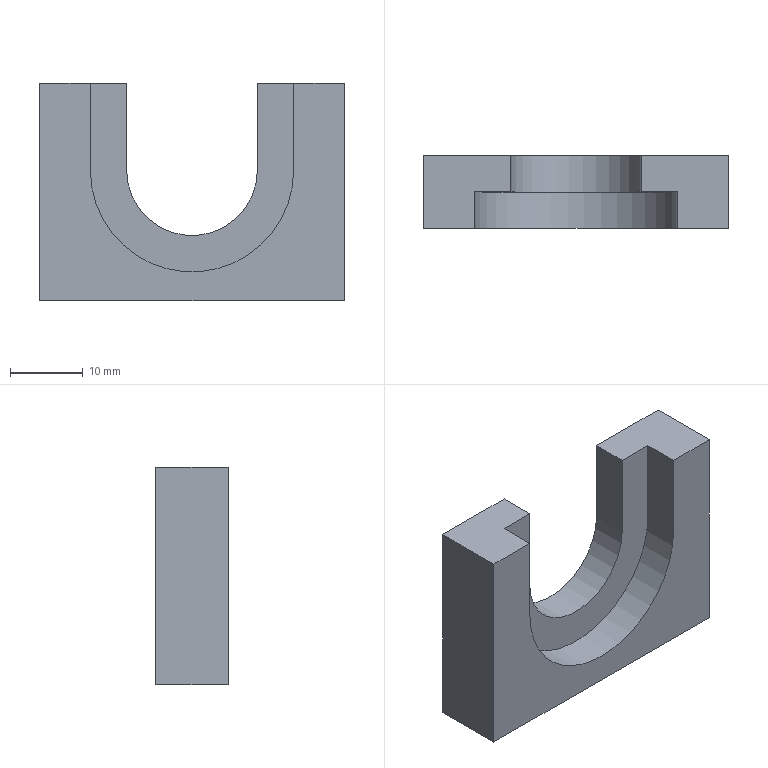Part | NX | features M5 六角凹头螺钉的柱形沉头孔1 2 | 1 solid | 14 faces | box 42 x 10 x 30 mm | volume 7664 mm3 | plane 12 | cylinder 2 | commonest cylinder face diameters 18 x1 28 x1
STEP:
#1=CARTESIAN_POINT('',(-9.,206.666,138.381));
#2=VERTEX_POINT('',#1);
#3=CARTESIAN_POINT('',(-9.,206.666,150.381));
#4=VERTEX_POINT('',#3);
#5=CARTESIAN_POINT('',(-9.,206.666,138.381));
#6=DIRECTION('',(0.,0.,1.));
#7=VECTOR('',#6,1000.);
#8=LINE('',#5,#7);
#9=EDGE_CURVE('',#2,#4,#8,.T.);
#10=ORIENTED_EDGE('',*,*,#9,.F.);
#11=CARTESIAN_POINT('',(-9.,211.666,138.381));
#12=VERTEX_POINT('',#11);
#13=CARTESIAN_POINT('',(-9.,214.666,138.381));
#14=DIRECTION('',(0.,-1.,0.));
#15=VECTOR('',#14,1000.);
#16=LINE('',#13,#15);
#17=EDGE_CURVE('',#12,#2,#16,.T.);
#18=ORIENTED_EDGE('',*,*,#17,.F.);
#19=CARTESIAN_POINT('',(-9.,211.666,150.381));
#20=VERTEX_POINT('',#19);
#21=CARTESIAN_POINT('',(-9.,211.666,135.381));
#22=DIRECTION('',(0.,0.,1.));
#23=VECTOR('',#22,1000.);
#24=LINE('',#21,#23);
#25=EDGE_CURVE('',#12,#20,#24,.T.);
#26=ORIENTED_EDGE('',*,*,#25,.T.);
#27=CARTESIAN_POINT('',(-9.,201.666,150.381));
#28=DIRECTION('',(0.,1.,0.));
#29=VECTOR('',#28,1000.);
#30=LINE('',#27,#29);
#31=EDGE_CURVE('',#4,#20,#30,.T.);
#32=ORIENTED_EDGE('',*,*,#31,.F.);
#33=EDGE_LOOP('',(#10,#18,#26,#32));
#34=FACE_BOUND('',#33,.T.);
#35=CARTESIAN_POINT('',(-9.,214.666,138.381));
#36=DIRECTION('',(-1.,0.,0.));
#37=DIRECTION('',(0.,0.,1.));
#38=AXIS2_PLACEMENT_3D('',#35,#36,#37);
#39=PLANE('',#38);
#40=ADVANCED_FACE('',(#34),#39,.F.);
#41=CARTESIAN_POINT('',(9.,206.666,150.381));
#42=VERTEX_POINT('',#41);
#43=CARTESIAN_POINT('',(9.,206.666,138.381));
#44=VERTEX_POINT('',#43);
#45=CARTESIAN_POINT('',(9.,206.666,138.381));
#46=DIRECTION('',(0.,0.,-1.));
#47=VECTOR('',#46,1000.);
#48=LINE('',#45,#47);
#49=EDGE_CURVE('',#42,#44,#48,.T.);
#50=ORIENTED_EDGE('',*,*,#49,.F.);
#51=CARTESIAN_POINT('',(9.,211.666,150.381));
#52=VERTEX_POINT('',#51);
#53=CARTESIAN_POINT('',(9.,201.666,150.381));
#54=DIRECTION('',(0.,-1.,0.));
#55=VECTOR('',#54,1000.);
#56=LINE('',#53,#55);
#57=EDGE_CURVE('',#52,#42,#56,.T.);
#58=ORIENTED_EDGE('',*,*,#57,.F.);
#59=CARTESIAN_POINT('',(9.,211.666,138.381));
#60=VERTEX_POINT('',#59);
#61=CARTESIAN_POINT('',(9.,211.666,138.381));
#62=DIRECTION('',(0.,0.,1.));
#63=VECTOR('',#62,1000.);
#64=LINE('',#61,#63);
#65=EDGE_CURVE('',#60,#52,#64,.T.);
#66=ORIENTED_EDGE('',*,*,#65,.F.);
#67=CARTESIAN_POINT('',(9.,214.666,138.381));
#68=DIRECTION('',(0.,-1.,0.));
#69=VECTOR('',#68,1000.);
#70=LINE('',#67,#69);
#71=EDGE_CURVE('',#60,#44,#70,.T.);
#72=ORIENTED_EDGE('',*,*,#71,.T.);
#73=EDGE_LOOP('',(#50,#58,#66,#72));
#74=FACE_BOUND('',#73,.T.);
#75=CARTESIAN_POINT('',(9.,214.666,138.381));
#76=DIRECTION('',(1.,0.,0.));
#77=DIRECTION('',(0.,1.,0.));
#78=AXIS2_PLACEMENT_3D('',#75,#76,#77);
#79=PLANE('',#78);
#80=ADVANCED_FACE('',(#74),#79,.F.);
#81=CARTESIAN_POINT('',(-0.000000942,206.666,138.381));
#82=DIRECTION('',(0.,1.,0.));
#83=DIRECTION('',(-1.,0.,0.));
#84=AXIS2_PLACEMENT_3D('',#81,#82,#83);
#85=CIRCLE('',#84,9.);
#86=EDGE_CURVE('',#44,#2,#85,.T.);
#87=ORIENTED_EDGE('',*,*,#86,.F.);
#88=ORIENTED_EDGE('',*,*,#71,.F.);
#89=CARTESIAN_POINT('',(-0.000000942,211.666,138.381));
#90=DIRECTION('',(0.,-1.,0.));
#91=DIRECTION('',(-1.,0.,0.));
#92=AXIS2_PLACEMENT_3D('',#89,#90,#91);
#93=CIRCLE('',#92,9.);
#94=EDGE_CURVE('',#12,#60,#93,.T.);
#95=ORIENTED_EDGE('',*,*,#94,.F.);
#96=ORIENTED_EDGE('',*,*,#17,.T.);
#97=EDGE_LOOP('',(#87,#88,#95,#96));
#98=FACE_BOUND('',#97,.T.);
#99=CARTESIAN_POINT('',(-0.000000942,214.666,138.381));
#100=DIRECTION('',(0.,-1.,0.));
#101=DIRECTION('',(1.,0.,0.));
#102=AXIS2_PLACEMENT_3D('',#99,#100,#101);
#103=CYLINDRICAL_SURFACE('',#102,9.);
#104=ADVANCED_FACE('',(#98),#103,.F.);
#105=CARTESIAN_POINT('',(-14.,201.666,150.381));
#106=VERTEX_POINT('',#105);
#107=CARTESIAN_POINT('',(-21.,201.666,150.381));
#108=VERTEX_POINT('',#107);
#109=CARTESIAN_POINT('',(30.,201.666,150.381));
#110=DIRECTION('',(-1.,0.,0.));
#111=VECTOR('',#110,1000.);
#112=LINE('',#109,#111);
#113=EDGE_CURVE('',#106,#108,#112,.T.);
#114=ORIENTED_EDGE('',*,*,#113,.F.);
#115=CARTESIAN_POINT('',(-14.,206.666,150.381));
#116=VERTEX_POINT('',#115);
#117=CARTESIAN_POINT('',(-14.,201.666,150.381));
#118=DIRECTION('',(0.,1.,0.));
#119=VECTOR('',#118,1000.);
#120=LINE('',#117,#119);
#121=EDGE_CURVE('',#106,#116,#120,.T.);
#122=ORIENTED_EDGE('',*,*,#121,.T.);
#123=CARTESIAN_POINT('',(30.,206.666,150.381));
#124=DIRECTION('',(-1.,0.,0.));
#125=VECTOR('',#124,1000.);
#126=LINE('',#123,#125);
#127=EDGE_CURVE('',#4,#116,#126,.T.);
#128=ORIENTED_EDGE('',*,*,#127,.F.);
#129=ORIENTED_EDGE('',*,*,#31,.T.);
#130=CARTESIAN_POINT('',(-21.,211.666,150.381));
#131=VERTEX_POINT('',#130);
#132=CARTESIAN_POINT('',(30.,211.666,150.381));
#133=DIRECTION('',(-1.,0.,0.));
#134=VECTOR('',#133,1000.);
#135=LINE('',#132,#134);
#136=EDGE_CURVE('',#20,#131,#135,.T.);
#137=ORIENTED_EDGE('',*,*,#136,.T.);
#138=CARTESIAN_POINT('',(-21.,137.875,150.381));
#139=DIRECTION('',(-0.000000003,1.,0.));
#140=VECTOR('',#139,1000.);
#141=LINE('',#138,#140);
#142=EDGE_CURVE('',#108,#131,#141,.T.);
#143=ORIENTED_EDGE('',*,*,#142,.F.);
#144=EDGE_LOOP('',(#114,#122,#128,#129,#137,#143));
#145=FACE_BOUND('',#144,.T.);
#146=CARTESIAN_POINT('',(30.,201.666,150.381));
#147=DIRECTION('',(0.,0.,-1.));
#148=DIRECTION('',(0.,1.,0.));
#149=AXIS2_PLACEMENT_3D('',#146,#147,#148);
#150=PLANE('',#149);
#151=ADVANCED_FACE('',(#145),#150,.F.);
#152=CARTESIAN_POINT('',(-21.,211.666,120.381));
#153=VERTEX_POINT('',#152);
#154=CARTESIAN_POINT('',(-21.,211.666,135.381));
#155=DIRECTION('',(-0.000000012,0.,-1.));
#156=VECTOR('',#155,1000.);
#157=LINE('',#154,#156);
#158=EDGE_CURVE('',#131,#153,#157,.T.);
#159=ORIENTED_EDGE('',*,*,#158,.T.);
#160=CARTESIAN_POINT('',(-21.,201.666,120.381));
#161=VERTEX_POINT('',#160);
#162=CARTESIAN_POINT('',(-21.,201.666,120.381));
#163=DIRECTION('',(-0.000000003,1.,0.));
#164=VECTOR('',#163,1000.);
#165=LINE('',#162,#164);
#166=EDGE_CURVE('',#161,#153,#165,.T.);
#167=ORIENTED_EDGE('',*,*,#166,.F.);
#168=CARTESIAN_POINT('',(-21.,201.666,135.381));
#169=DIRECTION('',(-0.000000012,0.,-1.));
#170=VECTOR('',#169,1000.);
#171=LINE('',#168,#170);
#172=EDGE_CURVE('',#108,#161,#171,.T.);
#173=ORIENTED_EDGE('',*,*,#172,.F.);
#174=ORIENTED_EDGE('',*,*,#142,.T.);
#175=EDGE_LOOP('',(#159,#167,#173,#174));
#176=FACE_BOUND('',#175,.T.);
#177=CARTESIAN_POINT('',(-21.,137.875,116.575));
#178=DIRECTION('',(1.,0.000000003,-0.000000012));
#179=DIRECTION('',(0.000000012,0.,1.));
#180=AXIS2_PLACEMENT_3D('',#177,#178,#179);
#181=PLANE('',#180);
#182=ADVANCED_FACE('',(#176),#181,.F.);
#183=CARTESIAN_POINT('',(21.,211.666,120.381));
#184=VERTEX_POINT('',#183);
#185=CARTESIAN_POINT('',(30.,211.666,120.381));
#186=DIRECTION('',(1.,0.,0.));
#187=VECTOR('',#186,1000.);
#188=LINE('',#185,#187);
#189=EDGE_CURVE('',#153,#184,#188,.T.);
#190=ORIENTED_EDGE('',*,*,#189,.T.);
#191=CARTESIAN_POINT('',(21.,201.666,120.381));
#192=VERTEX_POINT('',#191);
#193=CARTESIAN_POINT('',(21.,176.666,120.381));
#194=DIRECTION('',(0.,1.,0.));
#195=VECTOR('',#194,1000.);
#196=LINE('',#193,#195);
#197=EDGE_CURVE('',#192,#184,#196,.T.);
#198=ORIENTED_EDGE('',*,*,#197,.F.);
#199=CARTESIAN_POINT('',(30.,201.666,120.381));
#200=DIRECTION('',(1.,0.,0.));
#201=VECTOR('',#200,1000.);
#202=LINE('',#199,#201);
#203=EDGE_CURVE('',#161,#192,#202,.T.);
#204=ORIENTED_EDGE('',*,*,#203,.F.);
#205=ORIENTED_EDGE('',*,*,#166,.T.);
#206=EDGE_LOOP('',(#190,#198,#204,#205));
#207=FACE_BOUND('',#206,.T.);
#208=CARTESIAN_POINT('',(30.,201.666,120.381));
#209=DIRECTION('',(0.,0.,1.));
#210=DIRECTION('',(0.,-1.,0.));
#211=AXIS2_PLACEMENT_3D('',#208,#209,#210);
#212=PLANE('',#211);
#213=ADVANCED_FACE('',(#207),#212,.F.);
#214=CARTESIAN_POINT('',(21.,211.666,150.381));
#215=VERTEX_POINT('',#214);
#216=CARTESIAN_POINT('',(21.,211.666,135.381));
#217=DIRECTION('',(0.000000009,0.,1.));
#218=VECTOR('',#217,1000.);
#219=LINE('',#216,#218);
#220=EDGE_CURVE('',#184,#215,#219,.T.);
#221=ORIENTED_EDGE('',*,*,#220,.T.);
#222=CARTESIAN_POINT('',(21.,201.666,150.381));
#223=VERTEX_POINT('',#222);
#224=CARTESIAN_POINT('',(21.,201.666,150.381));
#225=DIRECTION('',(0.,1.,0.));
#226=VECTOR('',#225,1000.);
#227=LINE('',#224,#226);
#228=EDGE_CURVE('',#223,#215,#227,.T.);
#229=ORIENTED_EDGE('',*,*,#228,.F.);
#230=CARTESIAN_POINT('',(21.,201.666,135.381));
#231=DIRECTION('',(0.000000009,0.,1.));
#232=VECTOR('',#231,1000.);
#233=LINE('',#230,#232);
#234=EDGE_CURVE('',#192,#223,#233,.T.);
#235=ORIENTED_EDGE('',*,*,#234,.F.);
#236=ORIENTED_EDGE('',*,*,#197,.T.);
#237=EDGE_LOOP('',(#221,#229,#235,#236));
#238=FACE_BOUND('',#237,.T.);
#239=CARTESIAN_POINT('',(21.,176.666,126.866));
#240=DIRECTION('',(-1.,0.,0.000000009));
#241=DIRECTION('',(-0.000000009,0.,-1.));
#242=AXIS2_PLACEMENT_3D('',#239,#240,#241);
#243=PLANE('',#242);
#244=ADVANCED_FACE('',(#238),#243,.F.);
#245=CARTESIAN_POINT('',(14.,206.666,150.381));
#246=VERTEX_POINT('',#245);
#247=CARTESIAN_POINT('',(30.,206.666,150.381));
#248=DIRECTION('',(-1.,0.,0.));
#249=VECTOR('',#248,1000.);
#250=LINE('',#247,#249);
#251=EDGE_CURVE('',#246,#42,#250,.T.);
#252=ORIENTED_EDGE('',*,*,#251,.F.);
#253=CARTESIAN_POINT('',(14.,201.666,150.381));
#254=VERTEX_POINT('',#253);
#255=CARTESIAN_POINT('',(14.,201.666,150.381));
#256=DIRECTION('',(0.,-1.,0.));
#257=VECTOR('',#256,1000.);
#258=LINE('',#255,#257);
#259=EDGE_CURVE('',#246,#254,#258,.T.);
#260=ORIENTED_EDGE('',*,*,#259,.T.);
#261=CARTESIAN_POINT('',(30.,201.666,150.381));
#262=DIRECTION('',(-1.,0.,0.));
#263=VECTOR('',#262,1000.);
#264=LINE('',#261,#263);
#265=EDGE_CURVE('',#223,#254,#264,.T.);
#266=ORIENTED_EDGE('',*,*,#265,.F.);
#267=ORIENTED_EDGE('',*,*,#228,.T.);
#268=CARTESIAN_POINT('',(30.,211.666,150.381));
#269=DIRECTION('',(-1.,0.,0.));
#270=VECTOR('',#269,1000.);
#271=LINE('',#268,#270);
#272=EDGE_CURVE('',#215,#52,#271,.T.);
#273=ORIENTED_EDGE('',*,*,#272,.T.);
#274=ORIENTED_EDGE('',*,*,#57,.T.);
#275=EDGE_LOOP('',(#252,#260,#266,#267,#273,#274));
#276=FACE_BOUND('',#275,.T.);
#277=CARTESIAN_POINT('',(30.,201.666,150.381));
#278=DIRECTION('',(0.,0.,-1.));
#279=DIRECTION('',(0.,1.,0.));
#280=AXIS2_PLACEMENT_3D('',#277,#278,#279);
#281=PLANE('',#280);
#282=ADVANCED_FACE('',(#276),#281,.F.);
#283=CARTESIAN_POINT('',(-14.,201.666,138.381));
#284=VERTEX_POINT('',#283);
#285=CARTESIAN_POINT('',(14.,201.666,138.381));
#286=VERTEX_POINT('',#285);
#287=CARTESIAN_POINT('',(-0.000000942,201.666,138.381));
#288=DIRECTION('',(0.,-1.,0.));
#289=DIRECTION('',(-1.,0.,0.));
#290=AXIS2_PLACEMENT_3D('',#287,#288,#289);
#291=CIRCLE('',#290,14.);
#292=EDGE_CURVE('',#284,#286,#291,.T.);
#293=ORIENTED_EDGE('',*,*,#292,.F.);
#294=CARTESIAN_POINT('',(-14.,201.666,138.381));
#295=DIRECTION('',(0.,0.,-1.));
#296=VECTOR('',#295,1000.);
#297=LINE('',#294,#296);
#298=EDGE_CURVE('',#106,#284,#297,.T.);
#299=ORIENTED_EDGE('',*,*,#298,.F.);
#300=ORIENTED_EDGE('',*,*,#113,.T.);
#301=ORIENTED_EDGE('',*,*,#172,.T.);
#302=ORIENTED_EDGE('',*,*,#203,.T.);
#303=ORIENTED_EDGE('',*,*,#234,.T.);
#304=ORIENTED_EDGE('',*,*,#265,.T.);
#305=CARTESIAN_POINT('',(14.,201.666,138.381));
#306=DIRECTION('',(0.,0.,1.));
#307=VECTOR('',#306,1000.);
#308=LINE('',#305,#307);
#309=EDGE_CURVE('',#286,#254,#308,.T.);
#310=ORIENTED_EDGE('',*,*,#309,.F.);
#311=EDGE_LOOP('',(#293,#299,#300,#301,#302,#303,#304,#310));
#312=FACE_BOUND('',#311,.T.);
#313=CARTESIAN_POINT('',(-0.000000942,201.666,135.381));
#314=DIRECTION('',(0.,1.,0.));
#315=DIRECTION('',(-1.,0.,0.));
#316=AXIS2_PLACEMENT_3D('',#313,#314,#315);
#317=PLANE('',#316);
#318=ADVANCED_FACE('',(#312),#317,.F.);
#319=ORIENTED_EDGE('',*,*,#25,.F.);
#320=ORIENTED_EDGE('',*,*,#94,.T.);
#321=ORIENTED_EDGE('',*,*,#65,.T.);
#322=ORIENTED_EDGE('',*,*,#272,.F.);
#323=ORIENTED_EDGE('',*,*,#220,.F.);
#324=ORIENTED_EDGE('',*,*,#189,.F.);
#325=ORIENTED_EDGE('',*,*,#158,.F.);
#326=ORIENTED_EDGE('',*,*,#136,.F.);
#327=EDGE_LOOP('',(#319,#320,#321,#322,#323,#324,#325,#326));
#328=FACE_BOUND('',#327,.T.);
#329=CARTESIAN_POINT('',(-0.000000942,211.666,135.381));
#330=DIRECTION('',(0.,1.,0.));
#331=DIRECTION('',(-1.,0.,0.));
#332=AXIS2_PLACEMENT_3D('',#329,#330,#331);
#333=PLANE('',#332);
#334=ADVANCED_FACE('',(#328),#333,.T.);
#335=ORIENTED_EDGE('',*,*,#298,.T.);
#336=CARTESIAN_POINT('',(-14.,206.666,138.381));
#337=VERTEX_POINT('',#336);
#338=CARTESIAN_POINT('',(-14.,206.666,138.381));
#339=DIRECTION('',(0.,-1.,0.));
#340=VECTOR('',#339,1000.);
#341=LINE('',#338,#340);
#342=EDGE_CURVE('',#337,#284,#341,.T.);
#343=ORIENTED_EDGE('',*,*,#342,.F.);
#344=CARTESIAN_POINT('',(-14.,206.666,138.381));
#345=DIRECTION('',(0.,0.,-1.));
#346=VECTOR('',#345,1000.);
#347=LINE('',#344,#346);
#348=EDGE_CURVE('',#116,#337,#347,.T.);
#349=ORIENTED_EDGE('',*,*,#348,.F.);
#350=ORIENTED_EDGE('',*,*,#121,.F.);
#351=EDGE_LOOP('',(#335,#343,#349,#350));
#352=FACE_BOUND('',#351,.T.);
#353=CARTESIAN_POINT('',(-14.,206.666,138.381));
#354=DIRECTION('',(-1.,0.,0.));
#355=DIRECTION('',(0.,0.,1.));
#356=AXIS2_PLACEMENT_3D('',#353,#354,#355);
#357=PLANE('',#356);
#358=ADVANCED_FACE('',(#352),#357,.F.);
#359=CARTESIAN_POINT('',(14.,206.666,138.381));
#360=VERTEX_POINT('',#359);
#361=CARTESIAN_POINT('',(14.,206.666,138.381));
#362=DIRECTION('',(0.,0.,1.));
#363=VECTOR('',#362,1000.);
#364=LINE('',#361,#363);
#365=EDGE_CURVE('',#360,#246,#364,.T.);
#366=ORIENTED_EDGE('',*,*,#365,.F.);
#367=CARTESIAN_POINT('',(14.,206.666,138.381));
#368=DIRECTION('',(0.,-1.,0.));
#369=VECTOR('',#368,1000.);
#370=LINE('',#367,#369);
#371=EDGE_CURVE('',#360,#286,#370,.T.);
#372=ORIENTED_EDGE('',*,*,#371,.T.);
#373=ORIENTED_EDGE('',*,*,#309,.T.);
#374=ORIENTED_EDGE('',*,*,#259,.F.);
#375=EDGE_LOOP('',(#366,#372,#373,#374));
#376=FACE_BOUND('',#375,.T.);
#377=CARTESIAN_POINT('',(14.,206.666,138.381));
#378=DIRECTION('',(1.,0.,0.));
#379=DIRECTION('',(0.,0.,-1.));
#380=AXIS2_PLACEMENT_3D('',#377,#378,#379);
#381=PLANE('',#380);
#382=ADVANCED_FACE('',(#376),#381,.F.);
#383=ORIENTED_EDGE('',*,*,#127,.T.);
#384=ORIENTED_EDGE('',*,*,#348,.T.);
#385=CARTESIAN_POINT('',(-0.000000942,206.666,138.381));
#386=DIRECTION('',(0.,-1.,0.));
#387=DIRECTION('',(-1.,0.,0.));
#388=AXIS2_PLACEMENT_3D('',#385,#386,#387);
#389=CIRCLE('',#388,14.);
#390=EDGE_CURVE('',#337,#360,#389,.T.);
#391=ORIENTED_EDGE('',*,*,#390,.T.);
#392=ORIENTED_EDGE('',*,*,#365,.T.);
#393=ORIENTED_EDGE('',*,*,#251,.T.);
#394=ORIENTED_EDGE('',*,*,#49,.T.);
#395=ORIENTED_EDGE('',*,*,#86,.T.);
#396=ORIENTED_EDGE('',*,*,#9,.T.);
#397=EDGE_LOOP('',(#383,#384,#391,#392,#393,#394,#395,#396));
#398=FACE_BOUND('',#397,.T.);
#399=CARTESIAN_POINT('',(-0.000000942,206.666,138.381));
#400=DIRECTION('',(0.,-1.,0.));
#401=DIRECTION('',(1.,0.,0.));
#402=AXIS2_PLACEMENT_3D('',#399,#400,#401);
#403=PLANE('',#402);
#404=ADVANCED_FACE('',(#398),#403,.T.);
#405=ORIENTED_EDGE('',*,*,#292,.T.);
#406=ORIENTED_EDGE('',*,*,#371,.F.);
#407=ORIENTED_EDGE('',*,*,#390,.F.);
#408=ORIENTED_EDGE('',*,*,#342,.T.);
#409=EDGE_LOOP('',(#405,#406,#407,#408));
#410=FACE_BOUND('',#409,.T.);
#411=CARTESIAN_POINT('',(-0.000000942,206.666,138.381));
#412=DIRECTION('',(0.,-1.,0.));
#413=DIRECTION('',(1.,0.,0.));
#414=AXIS2_PLACEMENT_3D('',#411,#412,#413);
#415=CYLINDRICAL_SURFACE('',#414,14.);
#416=ADVANCED_FACE('',(#410),#415,.F.);
#417=CLOSED_SHELL('',(#40,#80,#104,#151,#182,#213,#244,#282,#318,#334,#358,#382,#404,#416));
#418=MANIFOLD_SOLID_BREP('',#417);
#419=(LENGTH_UNIT()NAMED_UNIT(*)SI_UNIT(.MILLI.,.METRE.));
#420=UNCERTAINTY_MEASURE_WITH_UNIT(LENGTH_MEASURE(0.00001),#419,'','');
#421=(NAMED_UNIT(*)PLANE_ANGLE_UNIT()SI_UNIT($,.RADIAN.));
#422=(NAMED_UNIT(*)SI_UNIT($,.STERADIAN.)SOLID_ANGLE_UNIT());
#423=(GEOMETRIC_REPRESENTATION_CONTEXT(3)GLOBAL_UNCERTAINTY_ASSIGNED_CONTEXT((#420))GLOBAL_UNIT_ASSIGNED_CONTEXT((#419,#421,#422))REPRESENTATION_CONTEXT('',''));
#424=ADVANCED_BREP_SHAPE_REPRESENTATION('',(#418),#423);